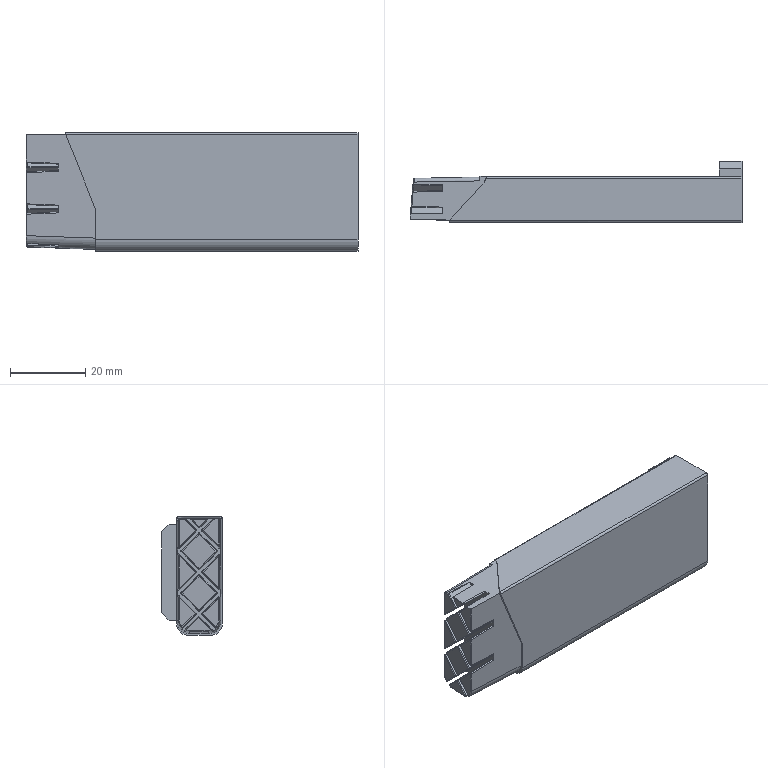Part | Creo | 1 solid | 206 faces | box 88.315 x 16.2 x 31.5 mm | volume 32634 mm3 | cylinder 71 | plane 66 | other 31 | sphere 30 | spline 8 | commonest cylinder face diameters 0.402 x61 1 x2 6 x2 6.03 x2 0.502 x1 2 x1